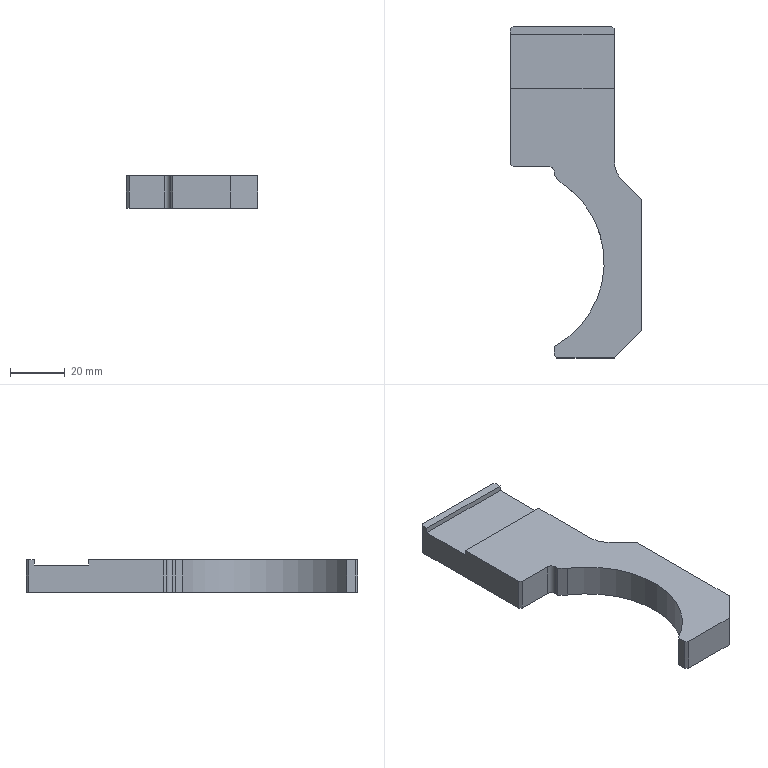Part | STEP file | 001-005-Shaft threading fixture adapter gripper | 1 solid | 24 faces | box 48 x 121.5 x 12 mm | volume 37787 mm3 | plane 21 | cylinder 3 | commonest cylinder face diameters 4 x1 20 x1 70 x1